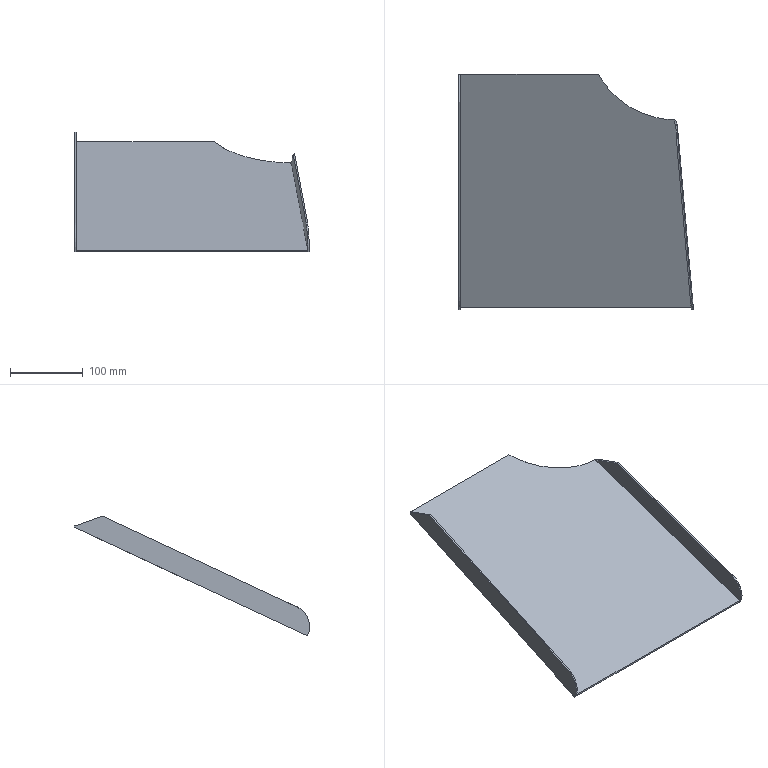Part | NX | features solid 2 | 1 solid | 20 faces | box 322.142 x 322.962 x 164.641 mm | volume 247812 mm3 | plane 10 | spline 9 | cylinder 1 | commonest cylinder face diameters 60 x1